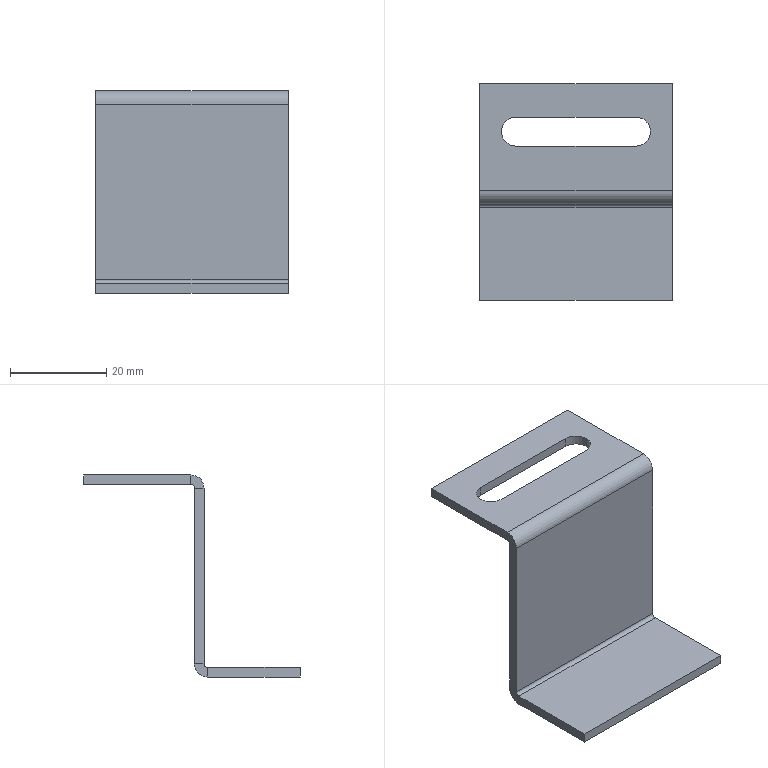Part | STEP file | PN_0022 sensor plate | 1 solid | 27 faces | box 40 x 45 x 42 mm | volume 6324 mm3 | plane 20 | cylinder 7 | commonest cylinder face diameters 6 x3 1.473 x2 5.473 x2